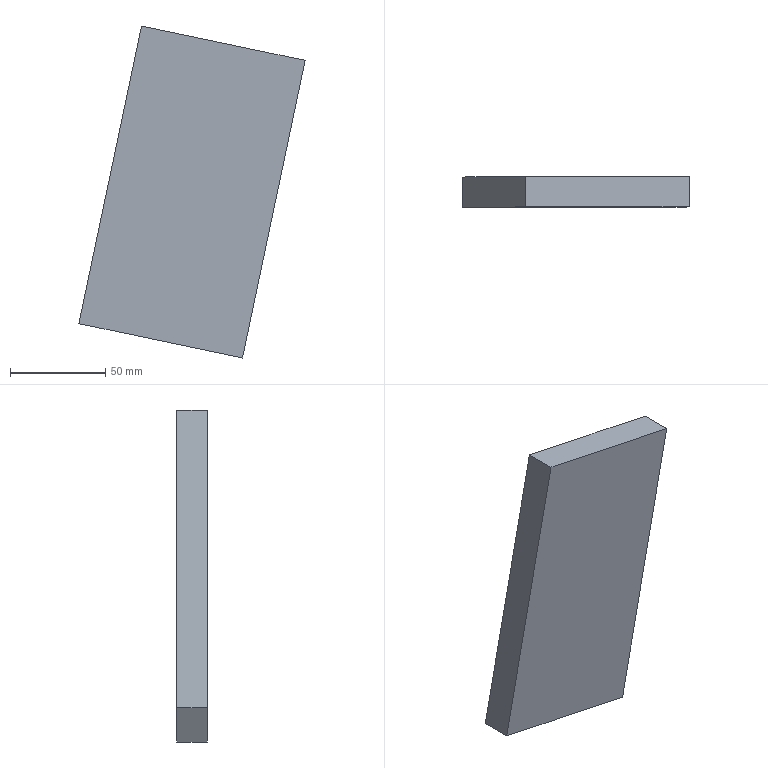Part | STEP file | 5_ESTAGIO_003-03 | 1 solid | 6 faces | box 119.022 x 16 x 174.677 mm | volume 225280 mm3 | plane 6
STEP:
#1=CARTESIAN_POINT('',(0.,0.,0.));
#2=DIRECTION('',(0.,0.,1.));
#3=DIRECTION('',(1.,0.,0.));
#4=AXIS2_PLACEMENT_3D('',#1,#2,#3);
#5=CARTESIAN_POINT('',(-2581.496,-875.15,1032.569));
#6=VERTEX_POINT('',#5);
#7=CARTESIAN_POINT('',(-2667.616,-875.15,1050.666));
#8=VERTEX_POINT('',#7);
#9=CARTESIAN_POINT('',(-2581.496,-875.15,1032.569));
#10=DIRECTION('',(-0.9786,0.,0.2056));
#11=VECTOR('',#10,1.);
#12=LINE('',#9,#11);
#13=CARTESIAN_POINT('',(-2581.496,-859.15,1032.569));
#14=DIRECTION('',(0.2056,0.,0.9786));
#15=DIRECTION('',(0.9786,0.,-0.2056));
#16=AXIS2_PLACEMENT_3D('',#13,#14,#15);
#17=PLANE('',#16);
#18=CARTESIAN_POINT('',(0.000000005,-16.));
#19=DIRECTION('',(-1.,0.));
#20=VECTOR('',#19,1.);
#21=LINE('',#18,#20);
#22=(GEOMETRIC_REPRESENTATION_CONTEXT(2)PARAMETRIC_REPRESENTATION_CONTEXT()REPRESENTATION_CONTEXT('',''));
#23=DEFINITIONAL_REPRESENTATION('',(#21),#22);
#24=PCURVE('',#17,#23);
#25=CARTESIAN_POINT('',(0.,-875.15,0.));
#26=DIRECTION('',(0.,1.,0.));
#27=DIRECTION('',(0.,0.,1.));
#28=AXIS2_PLACEMENT_3D('',#25,#26,#27);
#29=PLANE('',#28);
#30=CARTESIAN_POINT('',(1032.569,-2581.496));
#31=DIRECTION('',(0.2056,-0.9786));
#32=VECTOR('',#31,1.);
#33=LINE('',#30,#32);
#34=(GEOMETRIC_REPRESENTATION_CONTEXT(2)PARAMETRIC_REPRESENTATION_CONTEXT()REPRESENTATION_CONTEXT('',''));
#35=DEFINITIONAL_REPRESENTATION('',(#33),#34);
#36=PCURVE('',#29,#35);
#37=SURFACE_CURVE('',#12,(#24,#36),.PCURVE_S1.);
#38=EDGE_CURVE('',#6,#8,#37,.T.);
#39=ORIENTED_EDGE('',*,*,#38,.F.);
#40=CARTESIAN_POINT('',(-2581.496,-859.15,1032.569));
#41=VERTEX_POINT('',#40);
#42=CARTESIAN_POINT('',(-2581.496,-859.15,1032.569));
#43=DIRECTION('',(0.,-1.,0.));
#44=VECTOR('',#43,1.);
#45=LINE('',#42,#44);
#46=CARTESIAN_POINT('',(0.,0.));
#47=DIRECTION('',(0.,-1.));
#48=VECTOR('',#47,1.);
#49=LINE('',#46,#48);
#50=(GEOMETRIC_REPRESENTATION_CONTEXT(2)PARAMETRIC_REPRESENTATION_CONTEXT()REPRESENTATION_CONTEXT('',''));
#51=DEFINITIONAL_REPRESENTATION('',(#49),#50);
#52=PCURVE('',#17,#51);
#53=CARTESIAN_POINT('',(-2614.399,-859.15,875.989));
#54=DIRECTION('',(0.9786,0.,-0.2056));
#55=DIRECTION('',(-0.2056,0.,-0.9786));
#56=AXIS2_PLACEMENT_3D('',#53,#54,#55);
#57=PLANE('',#56);
#58=CARTESIAN_POINT('',(-160.,0.));
#59=DIRECTION('',(0.,-1.));
#60=VECTOR('',#59,1.);
#61=LINE('',#58,#60);
#62=(GEOMETRIC_REPRESENTATION_CONTEXT(2)PARAMETRIC_REPRESENTATION_CONTEXT()REPRESENTATION_CONTEXT('',''));
#63=DEFINITIONAL_REPRESENTATION('',(#61),#62);
#64=PCURVE('',#57,#63);
#65=SURFACE_CURVE('',#45,(#52,#64),.PCURVE_S1.);
#66=EDGE_CURVE('',#41,#6,#65,.T.);
#67=ORIENTED_EDGE('',*,*,#66,.F.);
#68=CARTESIAN_POINT('',(-2667.616,-859.15,1050.666));
#69=VERTEX_POINT('',#68);
#70=CARTESIAN_POINT('',(-2581.496,-859.15,1032.569));
#71=DIRECTION('',(-0.9786,0.,0.2056));
#72=VECTOR('',#71,1.);
#73=LINE('',#70,#72);
#74=CARTESIAN_POINT('',(0.000000005,0.));
#75=DIRECTION('',(-1.,0.));
#76=VECTOR('',#75,1.);
#77=LINE('',#74,#76);
#78=(GEOMETRIC_REPRESENTATION_CONTEXT(2)PARAMETRIC_REPRESENTATION_CONTEXT()REPRESENTATION_CONTEXT('',''));
#79=DEFINITIONAL_REPRESENTATION('',(#77),#78);
#80=PCURVE('',#17,#79);
#81=CARTESIAN_POINT('',(0.,-859.15,0.));
#82=DIRECTION('',(0.,1.,0.));
#83=DIRECTION('',(0.,0.,1.));
#84=AXIS2_PLACEMENT_3D('',#81,#82,#83);
#85=PLANE('',#84);
#86=CARTESIAN_POINT('',(1032.569,-2581.496));
#87=DIRECTION('',(0.2056,-0.9786));
#88=VECTOR('',#87,1.);
#89=LINE('',#86,#88);
#90=(GEOMETRIC_REPRESENTATION_CONTEXT(2)PARAMETRIC_REPRESENTATION_CONTEXT()REPRESENTATION_CONTEXT('',''));
#91=DEFINITIONAL_REPRESENTATION('',(#89),#90);
#92=PCURVE('',#85,#91);
#93=SURFACE_CURVE('',#73,(#80,#92),.PCURVE_S1.);
#94=EDGE_CURVE('',#41,#69,#93,.T.);
#95=ORIENTED_EDGE('',*,*,#94,.T.);
#96=CARTESIAN_POINT('',(-2667.616,-859.15,1050.666));
#97=DIRECTION('',(0.,-1.,0.));
#98=VECTOR('',#97,1.);
#99=LINE('',#96,#98);
#100=CARTESIAN_POINT('',(-88.,0.));
#101=DIRECTION('',(0.,-1.));
#102=VECTOR('',#101,1.);
#103=LINE('',#100,#102);
#104=(GEOMETRIC_REPRESENTATION_CONTEXT(2)PARAMETRIC_REPRESENTATION_CONTEXT()REPRESENTATION_CONTEXT('',''));
#105=DEFINITIONAL_REPRESENTATION('',(#103),#104);
#106=PCURVE('',#17,#105);
#107=CARTESIAN_POINT('',(-2667.616,-859.15,1050.666));
#108=DIRECTION('',(-0.9786,0.,0.2056));
#109=DIRECTION('',(0.2056,0.,0.9786));
#110=AXIS2_PLACEMENT_3D('',#107,#108,#109);
#111=PLANE('',#110);
#112=CARTESIAN_POINT('',(0.,0.));
#113=DIRECTION('',(0.,-1.));
#114=VECTOR('',#113,1.);
#115=LINE('',#112,#114);
#116=(GEOMETRIC_REPRESENTATION_CONTEXT(2)PARAMETRIC_REPRESENTATION_CONTEXT()REPRESENTATION_CONTEXT('',''));
#117=DEFINITIONAL_REPRESENTATION('',(#115),#116);
#118=PCURVE('',#111,#117);
#119=SURFACE_CURVE('',#99,(#106,#118),.PCURVE_S1.);
#120=EDGE_CURVE('',#69,#8,#119,.T.);
#121=ORIENTED_EDGE('',*,*,#120,.T.);
#122=EDGE_LOOP('',(#39,#67,#95,#121));
#123=FACE_BOUND('',#122,.T.);
#124=ADVANCED_FACE('',(#123),#17,.T.);
#125=CARTESIAN_POINT('',(-2614.399,-875.15,875.989));
#126=VERTEX_POINT('',#125);
#127=CARTESIAN_POINT('',(-2614.399,-875.15,875.989));
#128=DIRECTION('',(0.2056,0.,0.9786));
#129=VECTOR('',#128,1.);
#130=LINE('',#127,#129);
#131=CARTESIAN_POINT('',(0.,-16.));
#132=DIRECTION('',(-1.,0.));
#133=VECTOR('',#132,1.);
#134=LINE('',#131,#133);
#135=(GEOMETRIC_REPRESENTATION_CONTEXT(2)PARAMETRIC_REPRESENTATION_CONTEXT()REPRESENTATION_CONTEXT('',''));
#136=DEFINITIONAL_REPRESENTATION('',(#134),#135);
#137=PCURVE('',#57,#136);
#138=CARTESIAN_POINT('',(875.989,-2614.399));
#139=DIRECTION('',(0.9786,0.2056));
#140=VECTOR('',#139,1.);
#141=LINE('',#138,#140);
#142=(GEOMETRIC_REPRESENTATION_CONTEXT(2)PARAMETRIC_REPRESENTATION_CONTEXT()REPRESENTATION_CONTEXT('',''));
#143=DEFINITIONAL_REPRESENTATION('',(#141),#142);
#144=PCURVE('',#29,#143);
#145=SURFACE_CURVE('',#130,(#137,#144),.PCURVE_S1.);
#146=EDGE_CURVE('',#126,#6,#145,.T.);
#147=ORIENTED_EDGE('',*,*,#146,.F.);
#148=CARTESIAN_POINT('',(-2614.399,-859.15,875.989));
#149=VERTEX_POINT('',#148);
#150=CARTESIAN_POINT('',(-2614.399,-859.15,875.989));
#151=DIRECTION('',(0.,-1.,0.));
#152=VECTOR('',#151,1.);
#153=LINE('',#150,#152);
#154=CARTESIAN_POINT('',(0.,0.));
#155=DIRECTION('',(0.,-1.));
#156=VECTOR('',#155,1.);
#157=LINE('',#154,#156);
#158=(GEOMETRIC_REPRESENTATION_CONTEXT(2)PARAMETRIC_REPRESENTATION_CONTEXT()REPRESENTATION_CONTEXT('',''));
#159=DEFINITIONAL_REPRESENTATION('',(#157),#158);
#160=PCURVE('',#57,#159);
#161=CARTESIAN_POINT('',(-2700.519,-859.15,894.086));
#162=DIRECTION('',(-0.2056,0.,-0.9786));
#163=DIRECTION('',(-0.9786,0.,0.2056));
#164=AXIS2_PLACEMENT_3D('',#161,#162,#163);
#165=PLANE('',#164);
#166=CARTESIAN_POINT('',(-88.,0.));
#167=DIRECTION('',(0.,-1.));
#168=VECTOR('',#167,1.);
#169=LINE('',#166,#168);
#170=(GEOMETRIC_REPRESENTATION_CONTEXT(2)PARAMETRIC_REPRESENTATION_CONTEXT()REPRESENTATION_CONTEXT('',''));
#171=DEFINITIONAL_REPRESENTATION('',(#169),#170);
#172=PCURVE('',#165,#171);
#173=SURFACE_CURVE('',#153,(#160,#172),.PCURVE_S1.);
#174=EDGE_CURVE('',#149,#126,#173,.T.);
#175=ORIENTED_EDGE('',*,*,#174,.F.);
#176=CARTESIAN_POINT('',(-2614.399,-859.15,875.989));
#177=DIRECTION('',(0.2056,0.,0.9786));
#178=VECTOR('',#177,1.);
#179=LINE('',#176,#178);
#180=CARTESIAN_POINT('',(0.,0.));
#181=DIRECTION('',(-1.,0.));
#182=VECTOR('',#181,1.);
#183=LINE('',#180,#182);
#184=(GEOMETRIC_REPRESENTATION_CONTEXT(2)PARAMETRIC_REPRESENTATION_CONTEXT()REPRESENTATION_CONTEXT('',''));
#185=DEFINITIONAL_REPRESENTATION('',(#183),#184);
#186=PCURVE('',#57,#185);
#187=CARTESIAN_POINT('',(875.989,-2614.399));
#188=DIRECTION('',(0.9786,0.2056));
#189=VECTOR('',#188,1.);
#190=LINE('',#187,#189);
#191=(GEOMETRIC_REPRESENTATION_CONTEXT(2)PARAMETRIC_REPRESENTATION_CONTEXT()REPRESENTATION_CONTEXT('',''));
#192=DEFINITIONAL_REPRESENTATION('',(#190),#191);
#193=PCURVE('',#85,#192);
#194=SURFACE_CURVE('',#179,(#186,#193),.PCURVE_S1.);
#195=EDGE_CURVE('',#149,#41,#194,.T.);
#196=ORIENTED_EDGE('',*,*,#195,.T.);
#197=ORIENTED_EDGE('',*,*,#66,.T.);
#198=EDGE_LOOP('',(#147,#175,#196,#197));
#199=FACE_BOUND('',#198,.T.);
#200=ADVANCED_FACE('',(#199),#57,.T.);
#201=CARTESIAN_POINT('',(-2700.519,-875.15,894.086));
#202=VERTEX_POINT('',#201);
#203=CARTESIAN_POINT('',(-2700.519,-875.15,894.086));
#204=DIRECTION('',(0.9786,0.,-0.2056));
#205=VECTOR('',#204,1.);
#206=LINE('',#203,#205);
#207=CARTESIAN_POINT('',(0.,-16.));
#208=DIRECTION('',(-1.,0.));
#209=VECTOR('',#208,1.);
#210=LINE('',#207,#209);
#211=(GEOMETRIC_REPRESENTATION_CONTEXT(2)PARAMETRIC_REPRESENTATION_CONTEXT()REPRESENTATION_CONTEXT('',''));
#212=DEFINITIONAL_REPRESENTATION('',(#210),#211);
#213=PCURVE('',#165,#212);
#214=CARTESIAN_POINT('',(894.086,-2700.519));
#215=DIRECTION('',(-0.2056,0.9786));
#216=VECTOR('',#215,1.);
#217=LINE('',#214,#216);
#218=(GEOMETRIC_REPRESENTATION_CONTEXT(2)PARAMETRIC_REPRESENTATION_CONTEXT()REPRESENTATION_CONTEXT('',''));
#219=DEFINITIONAL_REPRESENTATION('',(#217),#218);
#220=PCURVE('',#29,#219);
#221=SURFACE_CURVE('',#206,(#213,#220),.PCURVE_S1.);
#222=EDGE_CURVE('',#202,#126,#221,.T.);
#223=ORIENTED_EDGE('',*,*,#222,.F.);
#224=CARTESIAN_POINT('',(-2700.519,-859.15,894.086));
#225=VERTEX_POINT('',#224);
#226=CARTESIAN_POINT('',(-2700.519,-859.15,894.086));
#227=DIRECTION('',(0.,-1.,0.));
#228=VECTOR('',#227,1.);
#229=LINE('',#226,#228);
#230=CARTESIAN_POINT('',(0.,0.));
#231=DIRECTION('',(0.,-1.));
#232=VECTOR('',#231,1.);
#233=LINE('',#230,#232);
#234=(GEOMETRIC_REPRESENTATION_CONTEXT(2)PARAMETRIC_REPRESENTATION_CONTEXT()REPRESENTATION_CONTEXT('',''));
#235=DEFINITIONAL_REPRESENTATION('',(#233),#234);
#236=PCURVE('',#165,#235);
#237=CARTESIAN_POINT('',(-160.,0.));
#238=DIRECTION('',(0.,-1.));
#239=VECTOR('',#238,1.);
#240=LINE('',#237,#239);
#241=(GEOMETRIC_REPRESENTATION_CONTEXT(2)PARAMETRIC_REPRESENTATION_CONTEXT()REPRESENTATION_CONTEXT('',''));
#242=DEFINITIONAL_REPRESENTATION('',(#240),#241);
#243=PCURVE('',#111,#242);
#244=SURFACE_CURVE('',#229,(#236,#243),.PCURVE_S1.);
#245=EDGE_CURVE('',#225,#202,#244,.T.);
#246=ORIENTED_EDGE('',*,*,#245,.F.);
#247=CARTESIAN_POINT('',(-2700.519,-859.15,894.086));
#248=DIRECTION('',(0.9786,0.,-0.2056));
#249=VECTOR('',#248,1.);
#250=LINE('',#247,#249);
#251=CARTESIAN_POINT('',(0.,0.));
#252=DIRECTION('',(-1.,0.));
#253=VECTOR('',#252,1.);
#254=LINE('',#251,#253);
#255=(GEOMETRIC_REPRESENTATION_CONTEXT(2)PARAMETRIC_REPRESENTATION_CONTEXT()REPRESENTATION_CONTEXT('',''));
#256=DEFINITIONAL_REPRESENTATION('',(#254),#255);
#257=PCURVE('',#165,#256);
#258=CARTESIAN_POINT('',(894.086,-2700.519));
#259=DIRECTION('',(-0.2056,0.9786));
#260=VECTOR('',#259,1.);
#261=LINE('',#258,#260);
#262=(GEOMETRIC_REPRESENTATION_CONTEXT(2)PARAMETRIC_REPRESENTATION_CONTEXT()REPRESENTATION_CONTEXT('',''));
#263=DEFINITIONAL_REPRESENTATION('',(#261),#262);
#264=PCURVE('',#85,#263);
#265=SURFACE_CURVE('',#250,(#257,#264),.PCURVE_S1.);
#266=EDGE_CURVE('',#225,#149,#265,.T.);
#267=ORIENTED_EDGE('',*,*,#266,.T.);
#268=ORIENTED_EDGE('',*,*,#174,.T.);
#269=EDGE_LOOP('',(#223,#246,#267,#268));
#270=FACE_BOUND('',#269,.T.);
#271=ADVANCED_FACE('',(#270),#165,.T.);
#272=CARTESIAN_POINT('',(-2667.616,-875.15,1050.666));
#273=DIRECTION('',(-0.2056,0.,-0.9786));
#274=VECTOR('',#273,1.);
#275=LINE('',#272,#274);
#276=CARTESIAN_POINT('',(-0.000000001,-16.));
#277=DIRECTION('',(-1.,0.));
#278=VECTOR('',#277,1.);
#279=LINE('',#276,#278);
#280=(GEOMETRIC_REPRESENTATION_CONTEXT(2)PARAMETRIC_REPRESENTATION_CONTEXT()REPRESENTATION_CONTEXT('',''));
#281=DEFINITIONAL_REPRESENTATION('',(#279),#280);
#282=PCURVE('',#111,#281);
#283=CARTESIAN_POINT('',(1050.666,-2667.616));
#284=DIRECTION('',(-0.9786,-0.2056));
#285=VECTOR('',#284,1.);
#286=LINE('',#283,#285);
#287=(GEOMETRIC_REPRESENTATION_CONTEXT(2)PARAMETRIC_REPRESENTATION_CONTEXT()REPRESENTATION_CONTEXT('',''));
#288=DEFINITIONAL_REPRESENTATION('',(#286),#287);
#289=PCURVE('',#29,#288);
#290=SURFACE_CURVE('',#275,(#282,#289),.PCURVE_S1.);
#291=EDGE_CURVE('',#8,#202,#290,.T.);
#292=ORIENTED_EDGE('',*,*,#291,.F.);
#293=ORIENTED_EDGE('',*,*,#120,.F.);
#294=CARTESIAN_POINT('',(-2667.616,-859.15,1050.666));
#295=DIRECTION('',(-0.2056,0.,-0.9786));
#296=VECTOR('',#295,1.);
#297=LINE('',#294,#296);
#298=CARTESIAN_POINT('',(-0.000000001,0.));
#299=DIRECTION('',(-1.,0.));
#300=VECTOR('',#299,1.);
#301=LINE('',#298,#300);
#302=(GEOMETRIC_REPRESENTATION_CONTEXT(2)PARAMETRIC_REPRESENTATION_CONTEXT()REPRESENTATION_CONTEXT('',''));
#303=DEFINITIONAL_REPRESENTATION('',(#301),#302);
#304=PCURVE('',#111,#303);
#305=CARTESIAN_POINT('',(1050.666,-2667.616));
#306=DIRECTION('',(-0.9786,-0.2056));
#307=VECTOR('',#306,1.);
#308=LINE('',#305,#307);
#309=(GEOMETRIC_REPRESENTATION_CONTEXT(2)PARAMETRIC_REPRESENTATION_CONTEXT()REPRESENTATION_CONTEXT('',''));
#310=DEFINITIONAL_REPRESENTATION('',(#308),#309);
#311=PCURVE('',#85,#310);
#312=SURFACE_CURVE('',#297,(#304,#311),.PCURVE_S1.);
#313=EDGE_CURVE('',#69,#225,#312,.T.);
#314=ORIENTED_EDGE('',*,*,#313,.T.);
#315=ORIENTED_EDGE('',*,*,#245,.T.);
#316=EDGE_LOOP('',(#292,#293,#314,#315));
#317=FACE_BOUND('',#316,.T.);
#318=ADVANCED_FACE('',(#317),#111,.T.);
#319=ORIENTED_EDGE('',*,*,#94,.F.);
#320=ORIENTED_EDGE('',*,*,#195,.F.);
#321=ORIENTED_EDGE('',*,*,#266,.F.);
#322=ORIENTED_EDGE('',*,*,#313,.F.);
#323=EDGE_LOOP('',(#319,#320,#321,#322));
#324=FACE_BOUND('',#323,.T.);
#325=ADVANCED_FACE('',(#324),#85,.T.);
#326=ORIENTED_EDGE('',*,*,#291,.T.);
#327=ORIENTED_EDGE('',*,*,#222,.T.);
#328=ORIENTED_EDGE('',*,*,#146,.T.);
#329=ORIENTED_EDGE('',*,*,#38,.T.);
#330=EDGE_LOOP('',(#326,#327,#328,#329));
#331=FACE_BOUND('',#330,.T.);
#332=ADVANCED_FACE('',(#331),#29,.F.);
#333=CLOSED_SHELL('',(#124,#200,#271,#318,#325,#332));
#334=MANIFOLD_SOLID_BREP('',#333);
#335=(LENGTH_UNIT()NAMED_UNIT(*)SI_UNIT(.MILLI.,.METRE.));
#336=UNCERTAINTY_MEASURE_WITH_UNIT(LENGTH_MEASURE(0.0000001),#335,'','');
#337=(NAMED_UNIT(*)PLANE_ANGLE_UNIT()SI_UNIT($,.RADIAN.));
#338=(NAMED_UNIT(*)SI_UNIT($,.STERADIAN.)SOLID_ANGLE_UNIT());
#339=(GEOMETRIC_REPRESENTATION_CONTEXT(3)GLOBAL_UNCERTAINTY_ASSIGNED_CONTEXT((#336))GLOBAL_UNIT_ASSIGNED_CONTEXT((#335,#337,#338))REPRESENTATION_CONTEXT('',''));
#340=ADVANCED_BREP_SHAPE_REPRESENTATION('',(#4,#334),#339);